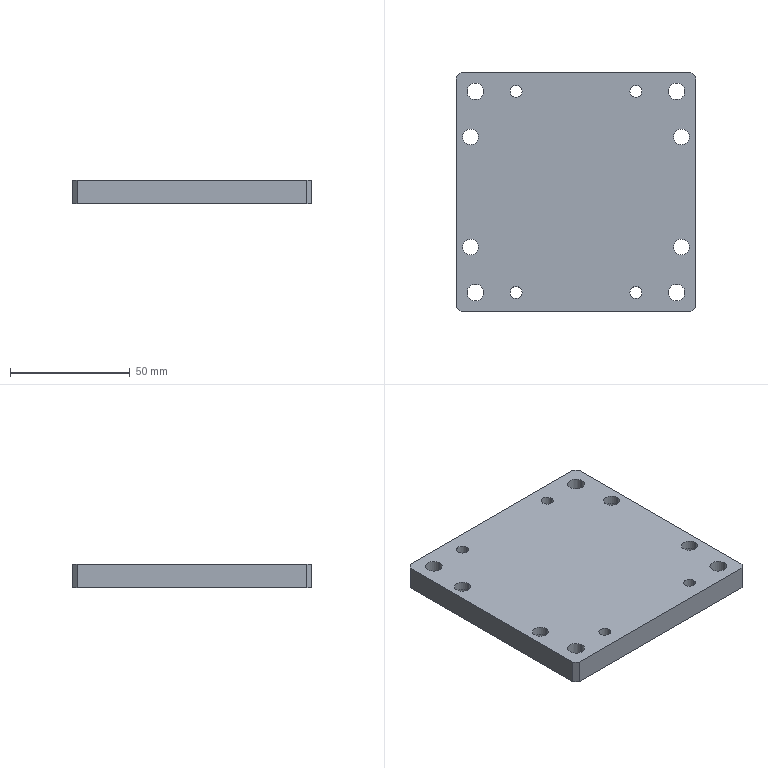Part | STEP file | PN_0038 vibratory adjusting plate A | 1 solid | 46 faces | box 100 x 100 x 10 mm | volume 94670 mm3 | cylinder 32 | plane 14 | commonest cylinder face diameters 5 x8 6.6 x8 7 x8 11 x8